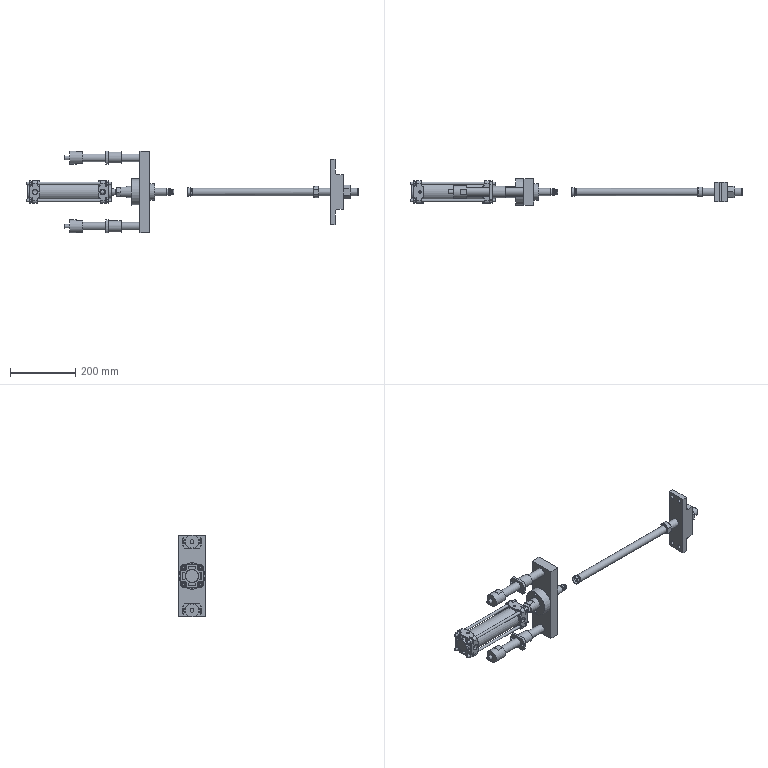Part | NX | features Hexagon Nut ISO - 4034 - M24 - N_Hexagon Nut ISO - 4034 - M24 - N 2, Hydraulic support1 2, Hydraulic support2 2, Hydraulic2.1_50 2, Hydraulic2.2_50 2, Hydraulic2.3_M18X1.5 2, Part2 2, bushing 2, clamp shaft 2, clamp stopper 2, mandrel expand 2, pipe setelah expand 2, stopper pipe 2, stopper pipe support 2 | 17 solids | 588 faces | box 1014 x 80 x 250 mm | volume 2060226 mm3 | plane 321 | cylinder 193 | cone 59 | spline 10 | torus 5 | commonest cylinder face diameters 4 x34 6 x16 5 x12 8 x12 20 x11 18 x10